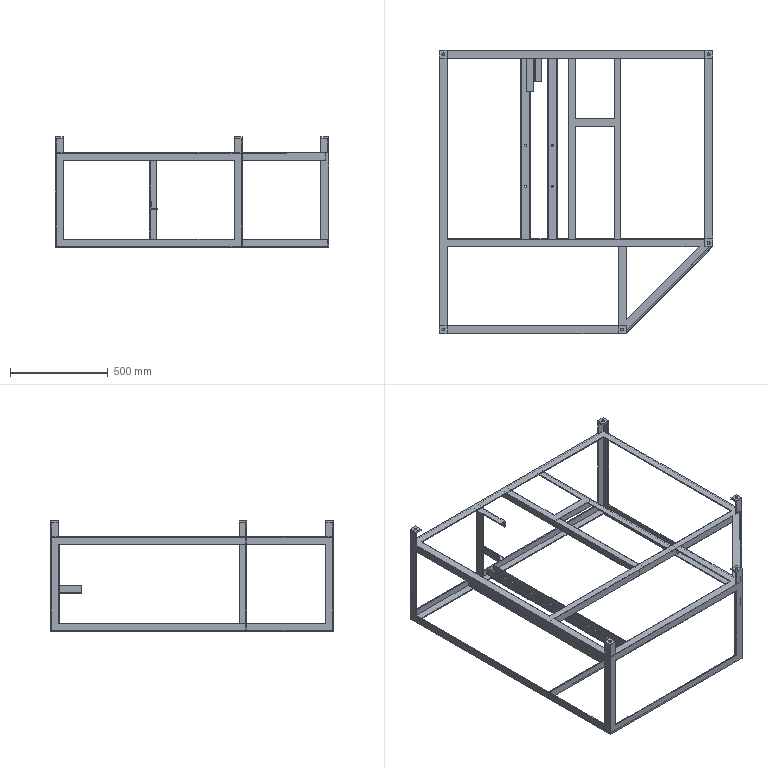Part | 1 solid | 193 faces | box 1400 x 1450 x 565 mm | volume 8315640 mm3 | plane 167 | cylinder 26 | commonest cylinder face diameters 14 x10 8.5 x8 10.2 x8